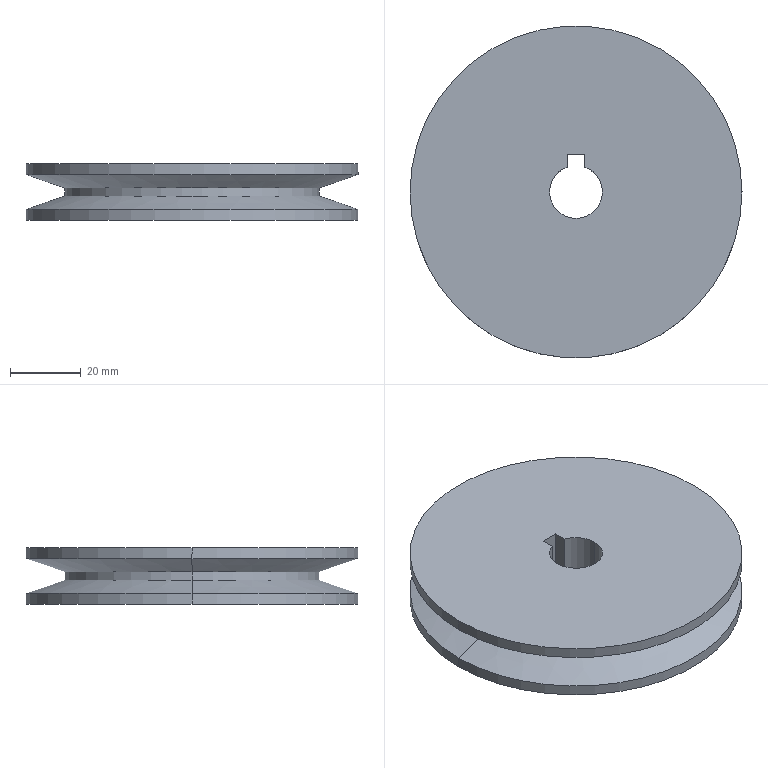Part | SolidWorks | features ICE 2, BaseBody 1 | 1 solid | 18 faces | box 94 x 94 x 16 mm | volume 89995 mm3 | cylinder 9 | plane 5 | cone 4 | commonest cylinder face diameters 94 x4 15 x3 72 x2
STEP:
#1=CARTESIAN_POINT('',(-7.5,0.,0.));
#2=VERTEX_POINT('',#1);
#3=CARTESIAN_POINT('',(7.5,0.,0.));
#4=VERTEX_POINT('',#3);
#5=CARTESIAN_POINT('',(0.,0.,0.));
#6=DIRECTION('',(0.,0.,1.));
#7=DIRECTION('',(1.,0.,0.));
#8=AXIS2_PLACEMENT_3D('',#5,#6,#7);
#9=CIRCLE('',#8,7.5);
#10=EDGE_CURVE('',#2,#4,#9,.T.);
#11=ORIENTED_EDGE('',*,*,#10,.F.);
#12=CARTESIAN_POINT('',(-7.5,0.,16.));
#13=VERTEX_POINT('',#12);
#14=CARTESIAN_POINT('',(-7.5,0.,0.));
#15=DIRECTION('',(0.,0.,1.));
#16=VECTOR('',#15,1000.);
#17=LINE('',#14,#16);
#18=EDGE_CURVE('',#2,#13,#17,.T.);
#19=ORIENTED_EDGE('',*,*,#18,.T.);
#20=CARTESIAN_POINT('',(7.5,0.,16.));
#21=VERTEX_POINT('',#20);
#22=CARTESIAN_POINT('',(0.,0.,16.));
#23=DIRECTION('',(0.,0.,1.));
#24=DIRECTION('',(1.,0.,0.));
#25=AXIS2_PLACEMENT_3D('',#22,#23,#24);
#26=CIRCLE('',#25,7.5);
#27=EDGE_CURVE('',#13,#21,#26,.T.);
#28=ORIENTED_EDGE('',*,*,#27,.T.);
#29=CARTESIAN_POINT('',(7.5,0.,0.));
#30=DIRECTION('',(0.,0.,1.));
#31=VECTOR('',#30,1000.);
#32=LINE('',#29,#31);
#33=EDGE_CURVE('',#4,#21,#32,.T.);
#34=ORIENTED_EDGE('',*,*,#33,.F.);
#35=EDGE_LOOP('',(#11,#19,#28,#34));
#36=FACE_OUTER_BOUND('',#35,.T.);
#37=CARTESIAN_POINT('',(0.,0.,0.));
#38=DIRECTION('',(0.,0.,1.));
#39=DIRECTION('',(1.,0.,0.));
#40=AXIS2_PLACEMENT_3D('',#37,#38,#39);
#41=CYLINDRICAL_SURFACE('',#40,7.5);
#42=ADVANCED_FACE('',(#36),#41,.F.);
#43=CARTESIAN_POINT('',(2.5,7.071,0.));
#44=VERTEX_POINT('',#43);
#45=CARTESIAN_POINT('',(0.,0.,0.));
#46=DIRECTION('',(0.,0.,1.));
#47=DIRECTION('',(1.,0.,0.));
#48=AXIS2_PLACEMENT_3D('',#45,#46,#47);
#49=CIRCLE('',#48,7.5);
#50=EDGE_CURVE('',#4,#44,#49,.T.);
#51=ORIENTED_EDGE('',*,*,#50,.F.);
#52=ORIENTED_EDGE('',*,*,#33,.T.);
#53=CARTESIAN_POINT('',(2.5,7.071,16.));
#54=VERTEX_POINT('',#53);
#55=CARTESIAN_POINT('',(0.,0.,16.));
#56=DIRECTION('',(0.,0.,1.));
#57=DIRECTION('',(1.,0.,0.));
#58=AXIS2_PLACEMENT_3D('',#55,#56,#57);
#59=CIRCLE('',#58,7.5);
#60=EDGE_CURVE('',#21,#54,#59,.T.);
#61=ORIENTED_EDGE('',*,*,#60,.T.);
#62=CARTESIAN_POINT('',(2.5,7.071,0.));
#63=DIRECTION('',(0.,0.,-1.));
#64=VECTOR('',#63,1000.);
#65=LINE('',#62,#64);
#66=EDGE_CURVE('',#54,#44,#65,.T.);
#67=ORIENTED_EDGE('',*,*,#66,.T.);
#68=EDGE_LOOP('',(#51,#52,#61,#67));
#69=FACE_OUTER_BOUND('',#68,.T.);
#70=CARTESIAN_POINT('',(0.,0.,0.));
#71=DIRECTION('',(0.,0.,1.));
#72=DIRECTION('',(1.,0.,0.));
#73=AXIS2_PLACEMENT_3D('',#70,#71,#72);
#74=CYLINDRICAL_SURFACE('',#73,7.5);
#75=ADVANCED_FACE('',(#69),#74,.F.);
#76=CARTESIAN_POINT('',(47.,0.,16.));
#77=VERTEX_POINT('',#76);
#78=CARTESIAN_POINT('',(-47.,0.,16.));
#79=VERTEX_POINT('',#78);
#80=CARTESIAN_POINT('',(0.,0.,16.));
#81=DIRECTION('',(0.,0.,1.));
#82=DIRECTION('',(-1.,0.,0.));
#83=AXIS2_PLACEMENT_3D('',#80,#81,#82);
#84=CIRCLE('',#83,47.);
#85=EDGE_CURVE('',#77,#79,#84,.T.);
#86=ORIENTED_EDGE('',*,*,#85,.F.);
#87=CARTESIAN_POINT('',(47.,0.,12.939));
#88=VERTEX_POINT('',#87);
#89=CARTESIAN_POINT('',(47.,0.,8.));
#90=DIRECTION('',(0.,0.,-1.));
#91=VECTOR('',#90,1000.);
#92=LINE('',#89,#91);
#93=EDGE_CURVE('',#77,#88,#92,.T.);
#94=ORIENTED_EDGE('',*,*,#93,.T.);
#95=CARTESIAN_POINT('',(-47.,0.,12.939));
#96=VERTEX_POINT('',#95);
#97=CARTESIAN_POINT('',(0.,0.,12.939));
#98=DIRECTION('',(0.,0.,1.));
#99=DIRECTION('',(-1.,0.,0.));
#100=AXIS2_PLACEMENT_3D('',#97,#98,#99);
#101=CIRCLE('',#100,47.);
#102=EDGE_CURVE('',#88,#96,#101,.T.);
#103=ORIENTED_EDGE('',*,*,#102,.T.);
#104=CARTESIAN_POINT('',(-47.,0.,8.));
#105=DIRECTION('',(0.,0.,-1.));
#106=VECTOR('',#105,1000.);
#107=LINE('',#104,#106);
#108=EDGE_CURVE('',#79,#96,#107,.T.);
#109=ORIENTED_EDGE('',*,*,#108,.F.);
#110=EDGE_LOOP('',(#86,#94,#103,#109));
#111=FACE_OUTER_BOUND('',#110,.T.);
#112=CARTESIAN_POINT('',(0.,0.,8.));
#113=DIRECTION('',(0.,0.,-1.));
#114=DIRECTION('',(-1.,0.,0.));
#115=AXIS2_PLACEMENT_3D('',#112,#113,#114);
#116=CYLINDRICAL_SURFACE('',#115,47.);
#117=ADVANCED_FACE('',(#111),#116,.T.);
#118=CARTESIAN_POINT('',(36.,0.,9.151));
#119=VERTEX_POINT('',#118);
#120=CARTESIAN_POINT('',(-36.,0.,9.151));
#121=VERTEX_POINT('',#120);
#122=CARTESIAN_POINT('',(0.,0.,9.151));
#123=DIRECTION('',(0.,0.,1.));
#124=DIRECTION('',(0.,1.,0.));
#125=AXIS2_PLACEMENT_3D('',#122,#123,#124);
#126=CIRCLE('',#125,36.);
#127=EDGE_CURVE('',#119,#121,#126,.T.);
#128=ORIENTED_EDGE('',*,*,#127,.T.);
#129=CARTESIAN_POINT('',(-47.,0.,12.939));
#130=DIRECTION('',(-0.9455,0.,0.3256));
#131=VECTOR('',#130,1000.);
#132=LINE('',#129,#131);
#133=EDGE_CURVE('',#121,#96,#132,.T.);
#134=ORIENTED_EDGE('',*,*,#133,.T.);
#135=ORIENTED_EDGE('',*,*,#102,.F.);
#136=CARTESIAN_POINT('',(47.,0.,12.939));
#137=DIRECTION('',(0.9455,0.,0.3256));
#138=VECTOR('',#137,1000.);
#139=LINE('',#136,#138);
#140=EDGE_CURVE('',#119,#88,#139,.T.);
#141=ORIENTED_EDGE('',*,*,#140,.F.);
#142=EDGE_LOOP('',(#128,#134,#135,#141));
#143=FACE_OUTER_BOUND('',#142,.T.);
#144=CARTESIAN_POINT('',(0.,0.,12.939));
#145=DIRECTION('',(0.,0.,1.));
#146=DIRECTION('',(1.,0.,0.));
#147=AXIS2_PLACEMENT_3D('',#144,#145,#146);
#148=CONICAL_SURFACE('',#147,47.,1.239);
#149=ADVANCED_FACE('',(#143),#148,.T.);
#150=CARTESIAN_POINT('',(36.,0.,6.849));
#151=VERTEX_POINT('',#150);
#152=CARTESIAN_POINT('',(-36.,0.,6.849));
#153=VERTEX_POINT('',#152);
#154=CARTESIAN_POINT('',(0.,0.,6.849));
#155=DIRECTION('',(0.,0.,1.));
#156=DIRECTION('',(1.,0.,0.));
#157=AXIS2_PLACEMENT_3D('',#154,#155,#156);
#158=CIRCLE('',#157,36.);
#159=EDGE_CURVE('',#151,#153,#158,.T.);
#160=ORIENTED_EDGE('',*,*,#159,.T.);
#161=CARTESIAN_POINT('',(-36.,0.,8.));
#162=DIRECTION('',(0.,0.,1.));
#163=VECTOR('',#162,1000.);
#164=LINE('',#161,#163);
#165=EDGE_CURVE('',#153,#121,#164,.T.);
#166=ORIENTED_EDGE('',*,*,#165,.T.);
#167=ORIENTED_EDGE('',*,*,#127,.F.);
#168=CARTESIAN_POINT('',(36.,0.,8.));
#169=DIRECTION('',(0.,0.,1.));
#170=VECTOR('',#169,1000.);
#171=LINE('',#168,#170);
#172=EDGE_CURVE('',#151,#119,#171,.T.);
#173=ORIENTED_EDGE('',*,*,#172,.F.);
#174=EDGE_LOOP('',(#160,#166,#167,#173));
#175=FACE_OUTER_BOUND('',#174,.T.);
#176=CARTESIAN_POINT('',(0.,0.,8.));
#177=DIRECTION('',(0.,0.,1.));
#178=DIRECTION('',(1.,0.,0.));
#179=AXIS2_PLACEMENT_3D('',#176,#177,#178);
#180=CYLINDRICAL_SURFACE('',#179,36.);
#181=ADVANCED_FACE('',(#175),#180,.T.);
#182=ORIENTED_EDGE('',*,*,#159,.F.);
#183=CARTESIAN_POINT('',(47.,0.,3.061));
#184=VERTEX_POINT('',#183);
#185=CARTESIAN_POINT('',(47.,0.,3.061));
#186=DIRECTION('',(0.9455,0.,-0.3256));
#187=VECTOR('',#186,1000.);
#188=LINE('',#185,#187);
#189=EDGE_CURVE('',#151,#184,#188,.T.);
#190=ORIENTED_EDGE('',*,*,#189,.T.);
#191=CARTESIAN_POINT('',(-47.,0.,3.061));
#192=VERTEX_POINT('',#191);
#193=CARTESIAN_POINT('',(0.,0.,3.061));
#194=DIRECTION('',(0.,0.,1.));
#195=DIRECTION('',(0.,1.,0.));
#196=AXIS2_PLACEMENT_3D('',#193,#194,#195);
#197=CIRCLE('',#196,47.);
#198=EDGE_CURVE('',#184,#192,#197,.T.);
#199=ORIENTED_EDGE('',*,*,#198,.T.);
#200=CARTESIAN_POINT('',(-47.,0.,3.061));
#201=DIRECTION('',(-0.9455,0.,-0.3256));
#202=VECTOR('',#201,1000.);
#203=LINE('',#200,#202);
#204=EDGE_CURVE('',#153,#192,#203,.T.);
#205=ORIENTED_EDGE('',*,*,#204,.F.);
#206=EDGE_LOOP('',(#182,#190,#199,#205));
#207=FACE_OUTER_BOUND('',#206,.T.);
#208=CARTESIAN_POINT('',(0.,0.,3.061));
#209=DIRECTION('',(0.,0.,-1.));
#210=DIRECTION('',(-1.,0.,0.));
#211=AXIS2_PLACEMENT_3D('',#208,#209,#210);
#212=CONICAL_SURFACE('',#211,47.,1.239);
#213=ADVANCED_FACE('',(#207),#212,.T.);
#214=ORIENTED_EDGE('',*,*,#198,.F.);
#215=CARTESIAN_POINT('',(47.,0.,0.));
#216=VERTEX_POINT('',#215);
#217=CARTESIAN_POINT('',(47.,0.,8.));
#218=DIRECTION('',(0.,0.,-1.));
#219=VECTOR('',#218,1000.);
#220=LINE('',#217,#219);
#221=EDGE_CURVE('',#184,#216,#220,.T.);
#222=ORIENTED_EDGE('',*,*,#221,.T.);
#223=CARTESIAN_POINT('',(-47.,0.,0.));
#224=VERTEX_POINT('',#223);
#225=CARTESIAN_POINT('',(0.,0.,0.));
#226=DIRECTION('',(0.,0.,1.));
#227=DIRECTION('',(-1.,0.,0.));
#228=AXIS2_PLACEMENT_3D('',#225,#226,#227);
#229=CIRCLE('',#228,47.);
#230=EDGE_CURVE('',#216,#224,#229,.T.);
#231=ORIENTED_EDGE('',*,*,#230,.T.);
#232=CARTESIAN_POINT('',(-47.,0.,8.));
#233=DIRECTION('',(0.,0.,-1.));
#234=VECTOR('',#233,1000.);
#235=LINE('',#232,#234);
#236=EDGE_CURVE('',#192,#224,#235,.T.);
#237=ORIENTED_EDGE('',*,*,#236,.F.);
#238=EDGE_LOOP('',(#214,#222,#231,#237));
#239=FACE_OUTER_BOUND('',#238,.T.);
#240=CARTESIAN_POINT('',(0.,0.,8.));
#241=DIRECTION('',(0.,0.,-1.));
#242=DIRECTION('',(-1.,0.,0.));
#243=AXIS2_PLACEMENT_3D('',#240,#241,#242);
#244=CYLINDRICAL_SURFACE('',#243,47.);
#245=ADVANCED_FACE('',(#239),#244,.T.);
#246=CARTESIAN_POINT('',(-2.5,10.7,16.));
#247=VERTEX_POINT('',#246);
#248=CARTESIAN_POINT('',(-2.5,7.071,16.));
#249=VERTEX_POINT('',#248);
#250=CARTESIAN_POINT('',(-2.5,10.7,16.));
#251=DIRECTION('',(0.,-1.,0.));
#252=VECTOR('',#251,1000.);
#253=LINE('',#250,#252);
#254=EDGE_CURVE('',#247,#249,#253,.T.);
#255=ORIENTED_EDGE('',*,*,#254,.F.);
#256=CARTESIAN_POINT('',(2.5,10.7,16.));
#257=VERTEX_POINT('',#256);
#258=CARTESIAN_POINT('',(-2.5,10.7,16.));
#259=DIRECTION('',(-1.,0.,0.));
#260=VECTOR('',#259,1000.);
#261=LINE('',#258,#260);
#262=EDGE_CURVE('',#257,#247,#261,.T.);
#263=ORIENTED_EDGE('',*,*,#262,.F.);
#264=CARTESIAN_POINT('',(2.5,10.7,16.));
#265=DIRECTION('',(0.,1.,0.));
#266=VECTOR('',#265,1000.);
#267=LINE('',#264,#266);
#268=EDGE_CURVE('',#54,#257,#267,.T.);
#269=ORIENTED_EDGE('',*,*,#268,.F.);
#270=ORIENTED_EDGE('',*,*,#60,.F.);
#271=ORIENTED_EDGE('',*,*,#27,.F.);
#272=CARTESIAN_POINT('',(0.,0.,16.));
#273=DIRECTION('',(0.,0.,1.));
#274=DIRECTION('',(1.,0.,0.));
#275=AXIS2_PLACEMENT_3D('',#272,#273,#274);
#276=CIRCLE('',#275,7.5);
#277=EDGE_CURVE('',#249,#13,#276,.T.);
#278=ORIENTED_EDGE('',*,*,#277,.F.);
#279=EDGE_LOOP('',(#255,#263,#269,#270,#271,#278));
#280=FACE_BOUND('',#279,.T.);
#281=CARTESIAN_POINT('',(0.,0.,16.));
#282=DIRECTION('',(0.,0.,1.));
#283=DIRECTION('',(-1.,0.,0.));
#284=AXIS2_PLACEMENT_3D('',#281,#282,#283);
#285=CIRCLE('',#284,47.);
#286=EDGE_CURVE('',#79,#77,#285,.T.);
#287=ORIENTED_EDGE('',*,*,#286,.T.);
#288=ORIENTED_EDGE('',*,*,#85,.T.);
#289=EDGE_LOOP('',(#287,#288));
#290=FACE_OUTER_BOUND('',#289,.T.);
#291=CARTESIAN_POINT('',(0.,23.5,16.));
#292=DIRECTION('',(0.,0.,1.));
#293=DIRECTION('',(1.,0.,0.));
#294=AXIS2_PLACEMENT_3D('',#291,#292,#293);
#295=PLANE('',#294);
#296=ADVANCED_FACE('',(#280,#290),#295,.T.);
#297=ORIENTED_EDGE('',*,*,#93,.F.);
#298=ORIENTED_EDGE('',*,*,#286,.F.);
#299=ORIENTED_EDGE('',*,*,#108,.T.);
#300=CARTESIAN_POINT('',(0.,0.,12.939));
#301=DIRECTION('',(0.,0.,1.));
#302=DIRECTION('',(-1.,0.,0.));
#303=AXIS2_PLACEMENT_3D('',#300,#301,#302);
#304=CIRCLE('',#303,47.);
#305=EDGE_CURVE('',#96,#88,#304,.T.);
#306=ORIENTED_EDGE('',*,*,#305,.T.);
#307=EDGE_LOOP('',(#297,#298,#299,#306));
#308=FACE_OUTER_BOUND('',#307,.T.);
#309=CARTESIAN_POINT('',(0.,0.,8.));
#310=DIRECTION('',(0.,0.,-1.));
#311=DIRECTION('',(-1.,0.,0.));
#312=AXIS2_PLACEMENT_3D('',#309,#310,#311);
#313=CYLINDRICAL_SURFACE('',#312,47.);
#314=ADVANCED_FACE('',(#308),#313,.T.);
#315=ORIENTED_EDGE('',*,*,#133,.F.);
#316=CARTESIAN_POINT('',(0.,0.,9.151));
#317=DIRECTION('',(0.,0.,1.));
#318=DIRECTION('',(0.,1.,0.));
#319=AXIS2_PLACEMENT_3D('',#316,#317,#318);
#320=CIRCLE('',#319,36.);
#321=EDGE_CURVE('',#121,#119,#320,.T.);
#322=ORIENTED_EDGE('',*,*,#321,.T.);
#323=ORIENTED_EDGE('',*,*,#140,.T.);
#324=ORIENTED_EDGE('',*,*,#305,.F.);
#325=EDGE_LOOP('',(#315,#322,#323,#324));
#326=FACE_OUTER_BOUND('',#325,.T.);
#327=CARTESIAN_POINT('',(0.,0.,12.939));
#328=DIRECTION('',(0.,0.,1.));
#329=DIRECTION('',(1.,0.,0.));
#330=AXIS2_PLACEMENT_3D('',#327,#328,#329);
#331=CONICAL_SURFACE('',#330,47.,1.239);
#332=ADVANCED_FACE('',(#326),#331,.T.);
#333=ORIENTED_EDGE('',*,*,#165,.F.);
#334=CARTESIAN_POINT('',(0.,0.,6.849));
#335=DIRECTION('',(0.,0.,1.));
#336=DIRECTION('',(1.,0.,0.));
#337=AXIS2_PLACEMENT_3D('',#334,#335,#336);
#338=CIRCLE('',#337,36.);
#339=EDGE_CURVE('',#153,#151,#338,.T.);
#340=ORIENTED_EDGE('',*,*,#339,.T.);
#341=ORIENTED_EDGE('',*,*,#172,.T.);
#342=ORIENTED_EDGE('',*,*,#321,.F.);
#343=EDGE_LOOP('',(#333,#340,#341,#342));
#344=FACE_OUTER_BOUND('',#343,.T.);
#345=CARTESIAN_POINT('',(0.,0.,8.));
#346=DIRECTION('',(0.,0.,1.));
#347=DIRECTION('',(1.,0.,0.));
#348=AXIS2_PLACEMENT_3D('',#345,#346,#347);
#349=CYLINDRICAL_SURFACE('',#348,36.);
#350=ADVANCED_FACE('',(#344),#349,.T.);
#351=ORIENTED_EDGE('',*,*,#189,.F.);
#352=ORIENTED_EDGE('',*,*,#339,.F.);
#353=ORIENTED_EDGE('',*,*,#204,.T.);
#354=CARTESIAN_POINT('',(0.,0.,3.061));
#355=DIRECTION('',(0.,0.,1.));
#356=DIRECTION('',(0.,1.,0.));
#357=AXIS2_PLACEMENT_3D('',#354,#355,#356);
#358=CIRCLE('',#357,47.);
#359=EDGE_CURVE('',#192,#184,#358,.T.);
#360=ORIENTED_EDGE('',*,*,#359,.T.);
#361=EDGE_LOOP('',(#351,#352,#353,#360));
#362=FACE_OUTER_BOUND('',#361,.T.);
#363=CARTESIAN_POINT('',(0.,0.,3.061));
#364=DIRECTION('',(0.,0.,-1.));
#365=DIRECTION('',(-1.,0.,0.));
#366=AXIS2_PLACEMENT_3D('',#363,#364,#365);
#367=CONICAL_SURFACE('',#366,47.,1.239);
#368=ADVANCED_FACE('',(#362),#367,.T.);
#369=ORIENTED_EDGE('',*,*,#221,.F.);
#370=ORIENTED_EDGE('',*,*,#359,.F.);
#371=ORIENTED_EDGE('',*,*,#236,.T.);
#372=CARTESIAN_POINT('',(0.,0.,0.));
#373=DIRECTION('',(0.,0.,1.));
#374=DIRECTION('',(-1.,0.,0.));
#375=AXIS2_PLACEMENT_3D('',#372,#373,#374);
#376=CIRCLE('',#375,47.);
#377=EDGE_CURVE('',#224,#216,#376,.T.);
#378=ORIENTED_EDGE('',*,*,#377,.T.);
#379=EDGE_LOOP('',(#369,#370,#371,#378));
#380=FACE_OUTER_BOUND('',#379,.T.);
#381=CARTESIAN_POINT('',(0.,0.,8.));
#382=DIRECTION('',(0.,0.,-1.));
#383=DIRECTION('',(-1.,0.,0.));
#384=AXIS2_PLACEMENT_3D('',#381,#382,#383);
#385=CYLINDRICAL_SURFACE('',#384,47.);
#386=ADVANCED_FACE('',(#380),#385,.T.);
#387=CARTESIAN_POINT('',(-2.5,10.7,0.));
#388=VERTEX_POINT('',#387);
#389=CARTESIAN_POINT('',(-2.5,7.071,0.));
#390=VERTEX_POINT('',#389);
#391=CARTESIAN_POINT('',(-2.5,10.7,0.));
#392=DIRECTION('',(0.,-1.,0.));
#393=VECTOR('',#392,1000.);
#394=LINE('',#391,#393);
#395=EDGE_CURVE('',#388,#390,#394,.T.);
#396=ORIENTED_EDGE('',*,*,#395,.T.);
#397=CARTESIAN_POINT('',(0.,0.,0.));
#398=DIRECTION('',(0.,0.,1.));
#399=DIRECTION('',(1.,0.,0.));
#400=AXIS2_PLACEMENT_3D('',#397,#398,#399);
#401=CIRCLE('',#400,7.5);
#402=EDGE_CURVE('',#390,#2,#401,.T.);
#403=ORIENTED_EDGE('',*,*,#402,.T.);
#404=ORIENTED_EDGE('',*,*,#10,.T.);
#405=ORIENTED_EDGE('',*,*,#50,.T.);
#406=CARTESIAN_POINT('',(2.5,10.7,0.));
#407=VERTEX_POINT('',#406);
#408=CARTESIAN_POINT('',(2.5,10.7,0.));
#409=DIRECTION('',(0.,1.,0.));
#410=VECTOR('',#409,1000.);
#411=LINE('',#408,#410);
#412=EDGE_CURVE('',#44,#407,#411,.T.);
#413=ORIENTED_EDGE('',*,*,#412,.T.);
#414=CARTESIAN_POINT('',(-2.5,10.7,0.));
#415=DIRECTION('',(-1.,0.,0.));
#416=VECTOR('',#415,1000.);
#417=LINE('',#414,#416);
#418=EDGE_CURVE('',#407,#388,#417,.T.);
#419=ORIENTED_EDGE('',*,*,#418,.T.);
#420=EDGE_LOOP('',(#396,#403,#404,#405,#413,#419));
#421=FACE_BOUND('',#420,.T.);
#422=ORIENTED_EDGE('',*,*,#377,.F.);
#423=ORIENTED_EDGE('',*,*,#230,.F.);
#424=EDGE_LOOP('',(#422,#423));
#425=FACE_OUTER_BOUND('',#424,.T.);
#426=CARTESIAN_POINT('',(0.,23.5,0.));
#427=DIRECTION('',(0.,0.,-1.));
#428=DIRECTION('',(-1.,0.,0.));
#429=AXIS2_PLACEMENT_3D('',#426,#427,#428);
#430=PLANE('',#429);
#431=ADVANCED_FACE('',(#421,#425),#430,.T.);
#432=ORIENTED_EDGE('',*,*,#18,.F.);
#433=ORIENTED_EDGE('',*,*,#402,.F.);
#434=CARTESIAN_POINT('',(-2.5,7.071,0.));
#435=DIRECTION('',(0.,0.,1.));
#436=VECTOR('',#435,1000.);
#437=LINE('',#434,#436);
#438=EDGE_CURVE('',#390,#249,#437,.T.);
#439=ORIENTED_EDGE('',*,*,#438,.T.);
#440=ORIENTED_EDGE('',*,*,#277,.T.);
#441=EDGE_LOOP('',(#432,#433,#439,#440));
#442=FACE_OUTER_BOUND('',#441,.T.);
#443=CARTESIAN_POINT('',(0.,0.,0.));
#444=DIRECTION('',(0.,0.,1.));
#445=DIRECTION('',(1.,0.,0.));
#446=AXIS2_PLACEMENT_3D('',#443,#444,#445);
#447=CYLINDRICAL_SURFACE('',#446,7.5);
#448=ADVANCED_FACE('',(#442),#447,.F.);
#449=ORIENTED_EDGE('',*,*,#395,.F.);
#450=CARTESIAN_POINT('',(-2.5,10.7,0.));
#451=DIRECTION('',(0.,0.,1.));
#452=VECTOR('',#451,1000.);
#453=LINE('',#450,#452);
#454=EDGE_CURVE('',#388,#247,#453,.T.);
#455=ORIENTED_EDGE('',*,*,#454,.T.);
#456=ORIENTED_EDGE('',*,*,#254,.T.);
#457=ORIENTED_EDGE('',*,*,#438,.F.);
#458=EDGE_LOOP('',(#449,#455,#456,#457));
#459=FACE_OUTER_BOUND('',#458,.T.);
#460=CARTESIAN_POINT('',(-2.5,10.7,0.));
#461=DIRECTION('',(-1.,0.,0.));
#462=DIRECTION('',(0.,-1.,0.));
#463=AXIS2_PLACEMENT_3D('',#460,#461,#462);
#464=PLANE('',#463);
#465=ADVANCED_FACE('',(#459),#464,.F.);
#466=ORIENTED_EDGE('',*,*,#268,.T.);
#467=CARTESIAN_POINT('',(2.5,10.7,0.));
#468=DIRECTION('',(0.,0.,1.));
#469=VECTOR('',#468,1000.);
#470=LINE('',#467,#469);
#471=EDGE_CURVE('',#407,#257,#470,.T.);
#472=ORIENTED_EDGE('',*,*,#471,.F.);
#473=ORIENTED_EDGE('',*,*,#412,.F.);
#474=ORIENTED_EDGE('',*,*,#66,.F.);
#475=EDGE_LOOP('',(#466,#472,#473,#474));
#476=FACE_OUTER_BOUND('',#475,.T.);
#477=CARTESIAN_POINT('',(2.5,10.7,0.));
#478=DIRECTION('',(1.,0.,0.));
#479=DIRECTION('',(0.,1.,0.));
#480=AXIS2_PLACEMENT_3D('',#477,#478,#479);
#481=PLANE('',#480);
#482=ADVANCED_FACE('',(#476),#481,.F.);
#483=ORIENTED_EDGE('',*,*,#262,.T.);
#484=ORIENTED_EDGE('',*,*,#454,.F.);
#485=ORIENTED_EDGE('',*,*,#418,.F.);
#486=ORIENTED_EDGE('',*,*,#471,.T.);
#487=EDGE_LOOP('',(#483,#484,#485,#486));
#488=FACE_OUTER_BOUND('',#487,.T.);
#489=CARTESIAN_POINT('',(-2.5,10.7,0.));
#490=DIRECTION('',(0.,1.,0.));
#491=DIRECTION('',(0.,0.,1.));
#492=AXIS2_PLACEMENT_3D('',#489,#490,#491);
#493=PLANE('',#492);
#494=ADVANCED_FACE('',(#488),#493,.F.);
#495=CLOSED_SHELL('',(#42,#75,#117,#149,#181,#213,#245,#296,#314,#332,#350,#368,#386,#431,#448,#465,#482,#494));
#496=MANIFOLD_SOLID_BREP('',#495);
#497=CARTESIAN_POINT('',(0.,0.,0.));
#498=DIRECTION('',(0.,0.,1.));
#499=DIRECTION('',(1.,0.,0.));
#500=AXIS2_PLACEMENT_3D('',#497,#498,#499);
#501=(LENGTH_UNIT()NAMED_UNIT(*)SI_UNIT(.MILLI.,.METRE.));
#502=UNCERTAINTY_MEASURE_WITH_UNIT(LENGTH_MEASURE(0.00001),#501,'','');
#503=(NAMED_UNIT(*)PLANE_ANGLE_UNIT()SI_UNIT($,.RADIAN.));
#504=(NAMED_UNIT(*)SI_UNIT($,.STERADIAN.)SOLID_ANGLE_UNIT());
#505=(GEOMETRIC_REPRESENTATION_CONTEXT(3)GLOBAL_UNCERTAINTY_ASSIGNED_CONTEXT((#502))GLOBAL_UNIT_ASSIGNED_CONTEXT((#501,#503,#504))REPRESENTATION_CONTEXT('',''));
#506=ADVANCED_BREP_SHAPE_REPRESENTATION('',(#496,#500),#505);